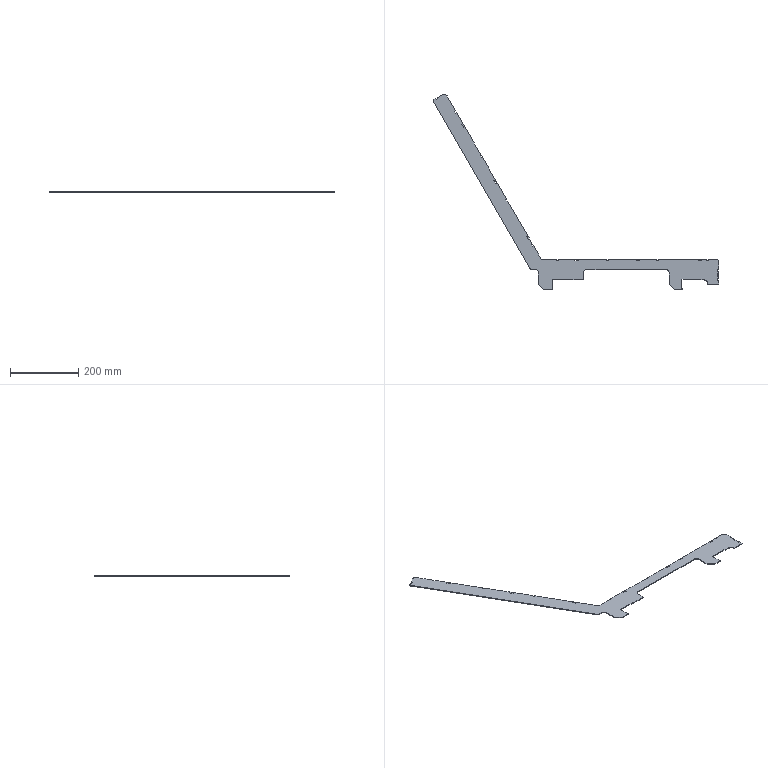Part | STEP file | zq001-2 | 1 solid | 110 faces | box 835.227 x 571.502 x 2 mm | volume 101233 mm3 | plane 102 | cylinder 8 | commonest cylinder face diameters 20 x7 8 x1